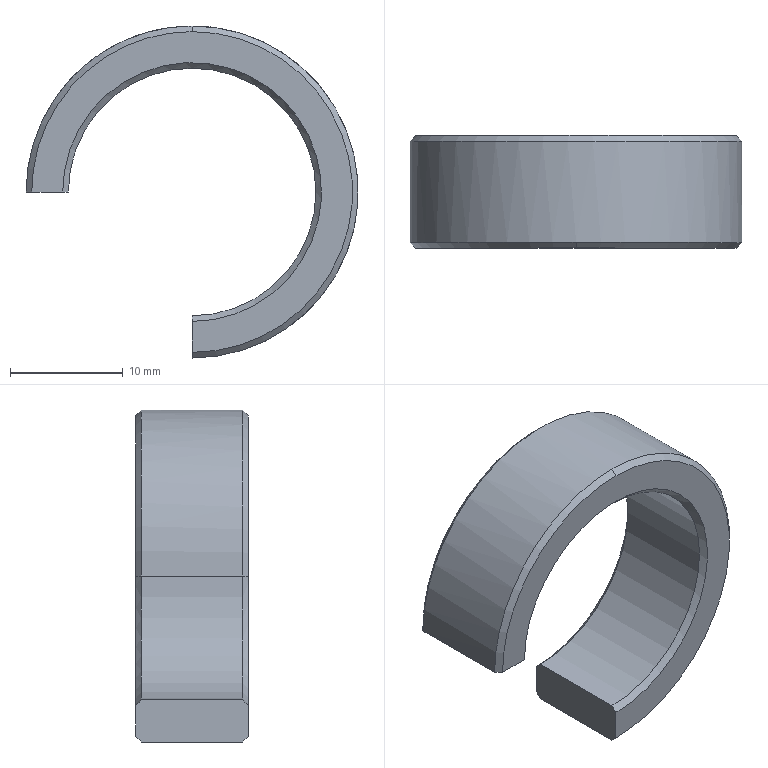Part | STEP file | Cuon T phu H01_3 | 1 solid | 12 faces | box 29.5 x 10 x 29.5 mm | volume 2245 mm3 | cone 6 | plane 4 | cylinder 2 | commonest cylinder face diameters 22 x1 29.5 x1
STEP:
#1=CARTESIAN_POINT('',(0.,0.,0.));
#2=DIRECTION('',(0.,0.,1.));
#3=DIRECTION('',(1.,0.,0.));
#4=AXIS2_PLACEMENT_3D('',#1,#2,#3);
#5=CARTESIAN_POINT('',(0.,10.,-11.5));
#6=VERTEX_POINT('',#5);
#7=CARTESIAN_POINT('',(0.,9.5,-11.));
#8=VERTEX_POINT('',#7);
#9=CARTESIAN_POINT('',(0.,-1.5,0.));
#10=DIRECTION('',(0.,-0.7071,0.7071));
#11=VECTOR('',#10,1.);
#12=LINE('',#9,#11);
#13=CARTESIAN_POINT('',(0.,9.5,0.));
#14=DIRECTION('',(0.,1.,0.));
#15=DIRECTION('',(0.,0.,1.));
#16=AXIS2_PLACEMENT_3D('',#13,#14,#15);
#17=CONICAL_SURFACE('',#16,11.,0.7854);
#18=CARTESIAN_POINT('',(3.142,-11.));
#19=DIRECTION('',(0.,-1.));
#20=VECTOR('',#19,1.);
#21=LINE('',#18,#20);
#22=(GEOMETRIC_REPRESENTATION_CONTEXT(2)PARAMETRIC_REPRESENTATION_CONTEXT()REPRESENTATION_CONTEXT('',''));
#23=DEFINITIONAL_REPRESENTATION('',(#21),#22);
#24=PCURVE('',#17,#23);
#25=CARTESIAN_POINT('',(0.,-63.834,33.935));
#26=DIRECTION('',(-1.,0.,0.));
#27=DIRECTION('',(0.,0.,1.));
#28=AXIS2_PLACEMENT_3D('',#25,#26,#27);
#29=PLANE('',#28);
#30=CARTESIAN_POINT('',(-33.935,62.334));
#31=DIRECTION('',(0.7071,-0.7071));
#32=VECTOR('',#31,1.);
#33=LINE('',#30,#32);
#34=(GEOMETRIC_REPRESENTATION_CONTEXT(2)PARAMETRIC_REPRESENTATION_CONTEXT()REPRESENTATION_CONTEXT('',''));
#35=DEFINITIONAL_REPRESENTATION('',(#33),#34);
#36=PCURVE('',#29,#35);
#37=SURFACE_CURVE('',#12,(#24,#36),.PCURVE_S1.);
#38=EDGE_CURVE('',#6,#8,#37,.T.);
#39=ORIENTED_EDGE('',*,*,#38,.F.);
#40=CARTESIAN_POINT('',(0.,10.,11.5));
#41=VERTEX_POINT('',#40);
#42=CARTESIAN_POINT('',(0.,10.,0.));
#43=DIRECTION('',(0.,-1.,0.));
#44=DIRECTION('',(0.,0.,1.));
#45=AXIS2_PLACEMENT_3D('',#42,#43,#44);
#46=CIRCLE('',#45,11.5);
#47=CARTESIAN_POINT('',(6.283,0.5));
#48=DIRECTION('',(-1.,0.));
#49=VECTOR('',#48,1.);
#50=LINE('',#47,#49);
#51=(GEOMETRIC_REPRESENTATION_CONTEXT(2)PARAMETRIC_REPRESENTATION_CONTEXT()REPRESENTATION_CONTEXT('',''));
#52=DEFINITIONAL_REPRESENTATION('',(#50),#51);
#53=PCURVE('',#17,#52);
#54=CARTESIAN_POINT('',(0.,10.,0.));
#55=DIRECTION('',(0.,1.,0.));
#56=DIRECTION('',(0.,0.,1.));
#57=AXIS2_PLACEMENT_3D('',#54,#55,#56);
#58=PLANE('',#57);
#59=CARTESIAN_POINT('',(11.5,0.));
#60=CARTESIAN_POINT('',(11.5,-19.919));
#61=CARTESIAN_POINT('',(-5.75,-9.959));
#62=CARTESIAN_POINT('',(-23.,0.));
#63=CARTESIAN_POINT('',(-5.75,9.959));
#64=CARTESIAN_POINT('',(11.5,19.919));
#65=CARTESIAN_POINT('',(11.5,0.));
#66=(BOUNDED_CURVE()B_SPLINE_CURVE(2,(#59,#60,#61,#62,#63,#64,#65),.UNSPECIFIED.,.T.,.F.)B_SPLINE_CURVE_WITH_KNOTS((1,2,2,2,2,1),(-2.094,0.,2.094,4.189,6.283,8.378),.UNSPECIFIED.)CURVE()GEOMETRIC_REPRESENTATION_ITEM()RATIONAL_B_SPLINE_CURVE((1.,0.5,1.,0.5,1.,0.5,1.))REPRESENTATION_ITEM(''));
#67=(GEOMETRIC_REPRESENTATION_CONTEXT(2)PARAMETRIC_REPRESENTATION_CONTEXT()REPRESENTATION_CONTEXT('',''));
#68=DEFINITIONAL_REPRESENTATION('',(#66),#67);
#69=PCURVE('',#58,#68);
#70=SURFACE_CURVE('',#46,(#53,#69),.PCURVE_S1.);
#71=EDGE_CURVE('',#6,#41,#70,.T.);
#72=ORIENTED_EDGE('',*,*,#71,.T.);
#73=CARTESIAN_POINT('',(0.,9.5,11.));
#74=VERTEX_POINT('',#73);
#75=CARTESIAN_POINT('',(0.,9.5,11.));
#76=DIRECTION('',(0.,0.7071,0.7071));
#77=VECTOR('',#76,1.);
#78=LINE('',#75,#77);
#79=CARTESIAN_POINT('',(0.,0.));
#80=DIRECTION('',(0.,1.));
#81=VECTOR('',#80,1.);
#82=LINE('',#79,#81);
#83=(GEOMETRIC_REPRESENTATION_CONTEXT(2)PARAMETRIC_REPRESENTATION_CONTEXT()REPRESENTATION_CONTEXT('',''));
#84=DEFINITIONAL_REPRESENTATION('',(#82),#83);
#85=PCURVE('',#17,#84);
#86=CARTESIAN_POINT('',(0.,9.5,0.));
#87=DIRECTION('',(0.,1.,0.));
#88=DIRECTION('',(0.,0.,1.));
#89=AXIS2_PLACEMENT_3D('',#86,#87,#88);
#90=CONICAL_SURFACE('',#89,11.,0.7854);
#91=CARTESIAN_POINT('',(6.283,0.));
#92=DIRECTION('',(0.,1.));
#93=VECTOR('',#92,1.);
#94=LINE('',#91,#93);
#95=(GEOMETRIC_REPRESENTATION_CONTEXT(2)PARAMETRIC_REPRESENTATION_CONTEXT()REPRESENTATION_CONTEXT('',''));
#96=DEFINITIONAL_REPRESENTATION('',(#94),#95);
#97=PCURVE('',#90,#96);
#98=SURFACE_CURVE('',#78,(#85,#97),.PCURVE_S1.);
#99=EDGE_CURVE('',#74,#41,#98,.T.);
#100=ORIENTED_EDGE('',*,*,#99,.F.);
#101=CARTESIAN_POINT('',(0.,9.5,0.));
#102=DIRECTION('',(0.,1.,0.));
#103=DIRECTION('',(0.,0.,1.));
#104=AXIS2_PLACEMENT_3D('',#101,#102,#103);
#105=CIRCLE('',#104,11.);
#106=CARTESIAN_POINT('',(0.,0.));
#107=DIRECTION('',(1.,0.));
#108=VECTOR('',#107,1.);
#109=LINE('',#106,#108);
#110=(GEOMETRIC_REPRESENTATION_CONTEXT(2)PARAMETRIC_REPRESENTATION_CONTEXT()REPRESENTATION_CONTEXT('',''));
#111=DEFINITIONAL_REPRESENTATION('',(#109),#110);
#112=PCURVE('',#17,#111);
#113=CARTESIAN_POINT('',(0.,10.,0.));
#114=DIRECTION('',(0.,-1.,0.));
#115=DIRECTION('',(0.,0.,-1.));
#116=AXIS2_PLACEMENT_3D('',#113,#114,#115);
#117=CYLINDRICAL_SURFACE('',#116,11.);
#118=CARTESIAN_POINT('',(3.142,0.5));
#119=DIRECTION('',(-1.,0.));
#120=VECTOR('',#119,1.);
#121=LINE('',#118,#120);
#122=(GEOMETRIC_REPRESENTATION_CONTEXT(2)PARAMETRIC_REPRESENTATION_CONTEXT()REPRESENTATION_CONTEXT('',''));
#123=DEFINITIONAL_REPRESENTATION('',(#121),#122);
#124=PCURVE('',#117,#123);
#125=SURFACE_CURVE('',#105,(#112,#124),.PCURVE_S1.);
#126=EDGE_CURVE('',#74,#8,#125,.T.);
#127=ORIENTED_EDGE('',*,*,#126,.T.);
#128=EDGE_LOOP('',(#39,#72,#100,#127));
#129=FACE_BOUND('',#128,.F.);
#130=ADVANCED_FACE('',(#129),#17,.F.);
#131=CARTESIAN_POINT('',(0.,0.,14.25));
#132=VERTEX_POINT('',#131);
#133=CARTESIAN_POINT('',(-14.25,0.,0.));
#134=VERTEX_POINT('',#133);
#135=CARTESIAN_POINT('',(0.,0.,0.));
#136=DIRECTION('',(0.,-1.,0.));
#137=DIRECTION('',(0.,0.,1.));
#138=AXIS2_PLACEMENT_3D('',#135,#136,#137);
#139=CIRCLE('',#138,14.25);
#140=CARTESIAN_POINT('',(0.,0.5,0.));
#141=DIRECTION('',(0.,1.,0.));
#142=DIRECTION('',(0.,0.,1.));
#143=AXIS2_PLACEMENT_3D('',#140,#141,#142);
#144=CONICAL_SURFACE('',#143,14.75,0.7854);
#145=CARTESIAN_POINT('',(6.283,-0.5));
#146=DIRECTION('',(-1.,0.));
#147=VECTOR('',#146,1.);
#148=LINE('',#145,#147);
#149=(GEOMETRIC_REPRESENTATION_CONTEXT(2)PARAMETRIC_REPRESENTATION_CONTEXT()REPRESENTATION_CONTEXT('',''));
#150=DEFINITIONAL_REPRESENTATION('',(#148),#149);
#151=PCURVE('',#144,#150);
#152=CARTESIAN_POINT('',(0.,0.,0.));
#153=DIRECTION('',(0.,1.,0.));
#154=DIRECTION('',(0.,0.,1.));
#155=AXIS2_PLACEMENT_3D('',#152,#153,#154);
#156=PLANE('',#155);
#157=CARTESIAN_POINT('',(14.25,0.));
#158=CARTESIAN_POINT('',(14.25,-24.682));
#159=CARTESIAN_POINT('',(-7.125,-12.341));
#160=CARTESIAN_POINT('',(-28.5,0.));
#161=CARTESIAN_POINT('',(-7.125,12.341));
#162=CARTESIAN_POINT('',(14.25,24.682));
#163=CARTESIAN_POINT('',(14.25,0.));
#164=(BOUNDED_CURVE()B_SPLINE_CURVE(2,(#157,#158,#159,#160,#161,#162,#163),.UNSPECIFIED.,.T.,.F.)B_SPLINE_CURVE_WITH_KNOTS((1,2,2,2,2,1),(-2.094,0.,2.094,4.189,6.283,8.378),.UNSPECIFIED.)CURVE()GEOMETRIC_REPRESENTATION_ITEM()RATIONAL_B_SPLINE_CURVE((1.,0.5,1.,0.5,1.,0.5,1.))REPRESENTATION_ITEM(''));
#165=(GEOMETRIC_REPRESENTATION_CONTEXT(2)PARAMETRIC_REPRESENTATION_CONTEXT()REPRESENTATION_CONTEXT('',''));
#166=DEFINITIONAL_REPRESENTATION('',(#164),#165);
#167=PCURVE('',#156,#166);
#168=SURFACE_CURVE('',#139,(#151,#167),.PCURVE_S1.);
#169=EDGE_CURVE('',#132,#134,#168,.T.);
#170=ORIENTED_EDGE('',*,*,#169,.F.);
#171=CARTESIAN_POINT('',(0.,0.5,14.75));
#172=VERTEX_POINT('',#171);
#173=CARTESIAN_POINT('',(0.,0.5,14.75));
#174=DIRECTION('',(0.,0.7071,0.7071));
#175=VECTOR('',#174,1.);
#176=LINE('',#173,#175);
#177=CARTESIAN_POINT('',(6.283,0.));
#178=DIRECTION('',(0.,1.));
#179=VECTOR('',#178,1.);
#180=LINE('',#177,#179);
#181=(GEOMETRIC_REPRESENTATION_CONTEXT(2)PARAMETRIC_REPRESENTATION_CONTEXT()REPRESENTATION_CONTEXT('',''));
#182=DEFINITIONAL_REPRESENTATION('',(#180),#181);
#183=PCURVE('',#144,#182);
#184=CARTESIAN_POINT('',(0.,0.5,0.));
#185=DIRECTION('',(0.,1.,0.));
#186=DIRECTION('',(0.,0.,1.));
#187=AXIS2_PLACEMENT_3D('',#184,#185,#186);
#188=CONICAL_SURFACE('',#187,14.75,0.7854);
#189=CARTESIAN_POINT('',(0.,0.));
#190=DIRECTION('',(0.,1.));
#191=VECTOR('',#190,1.);
#192=LINE('',#189,#191);
#193=(GEOMETRIC_REPRESENTATION_CONTEXT(2)PARAMETRIC_REPRESENTATION_CONTEXT()REPRESENTATION_CONTEXT('',''));
#194=DEFINITIONAL_REPRESENTATION('',(#192),#193);
#195=PCURVE('',#188,#194);
#196=SURFACE_CURVE('',#176,(#183,#195),.PCURVE_S1.);
#197=EDGE_CURVE('',#132,#172,#196,.T.);
#198=ORIENTED_EDGE('',*,*,#197,.T.);
#199=CARTESIAN_POINT('',(-14.75,0.5,0.));
#200=VERTEX_POINT('',#199);
#201=CARTESIAN_POINT('',(0.,0.5,0.));
#202=DIRECTION('',(0.,1.,0.));
#203=DIRECTION('',(0.,0.,1.));
#204=AXIS2_PLACEMENT_3D('',#201,#202,#203);
#205=CIRCLE('',#204,14.75);
#206=CARTESIAN_POINT('',(0.,0.));
#207=DIRECTION('',(1.,0.));
#208=VECTOR('',#207,1.);
#209=LINE('',#206,#208);
#210=(GEOMETRIC_REPRESENTATION_CONTEXT(2)PARAMETRIC_REPRESENTATION_CONTEXT()REPRESENTATION_CONTEXT('',''));
#211=DEFINITIONAL_REPRESENTATION('',(#209),#210);
#212=PCURVE('',#144,#211);
#213=CARTESIAN_POINT('',(0.,10.,0.));
#214=DIRECTION('',(0.,-1.,0.));
#215=DIRECTION('',(0.,0.,-1.));
#216=AXIS2_PLACEMENT_3D('',#213,#214,#215);
#217=CYLINDRICAL_SURFACE('',#216,14.75);
#218=CARTESIAN_POINT('',(9.425,9.5));
#219=DIRECTION('',(-1.,0.));
#220=VECTOR('',#219,1.);
#221=LINE('',#218,#220);
#222=(GEOMETRIC_REPRESENTATION_CONTEXT(2)PARAMETRIC_REPRESENTATION_CONTEXT()REPRESENTATION_CONTEXT('',''));
#223=DEFINITIONAL_REPRESENTATION('',(#221),#222);
#224=PCURVE('',#217,#223);
#225=SURFACE_CURVE('',#205,(#212,#224),.PCURVE_S1.);
#226=EDGE_CURVE('',#200,#172,#225,.T.);
#227=ORIENTED_EDGE('',*,*,#226,.F.);
#228=CARTESIAN_POINT('',(0.,-14.25,0.));
#229=DIRECTION('',(-0.7071,0.7071,0.));
#230=VECTOR('',#229,1.);
#231=LINE('',#228,#230);
#232=CARTESIAN_POINT('',(4.712,-14.75));
#233=DIRECTION('',(0.,1.));
#234=VECTOR('',#233,1.);
#235=LINE('',#232,#234);
#236=(GEOMETRIC_REPRESENTATION_CONTEXT(2)PARAMETRIC_REPRESENTATION_CONTEXT()REPRESENTATION_CONTEXT('',''));
#237=DEFINITIONAL_REPRESENTATION('',(#235),#236);
#238=PCURVE('',#144,#237);
#239=CARTESIAN_POINT('',(0.,-52.57,0.));
#240=DIRECTION('',(0.,0.,1.));
#241=DIRECTION('',(1.,0.,0.));
#242=AXIS2_PLACEMENT_3D('',#239,#240,#241);
#243=PLANE('',#242);
#244=CARTESIAN_POINT('',(0.,38.32));
#245=DIRECTION('',(-0.7071,0.7071));
#246=VECTOR('',#245,1.);
#247=LINE('',#244,#246);
#248=(GEOMETRIC_REPRESENTATION_CONTEXT(2)PARAMETRIC_REPRESENTATION_CONTEXT()REPRESENTATION_CONTEXT('',''));
#249=DEFINITIONAL_REPRESENTATION('',(#247),#248);
#250=PCURVE('',#243,#249);
#251=SURFACE_CURVE('',#231,(#238,#250),.PCURVE_S1.);
#252=EDGE_CURVE('',#134,#200,#251,.T.);
#253=ORIENTED_EDGE('',*,*,#252,.F.);
#254=EDGE_LOOP('',(#170,#198,#227,#253));
#255=FACE_BOUND('',#254,.T.);
#256=ADVANCED_FACE('',(#255),#144,.T.);
#257=CARTESIAN_POINT('',(-14.25,10.,0.));
#258=VERTEX_POINT('',#257);
#259=CARTESIAN_POINT('',(-11.5,10.,0.));
#260=VERTEX_POINT('',#259);
#261=CARTESIAN_POINT('',(0.,10.,0.));
#262=DIRECTION('',(1.,0.,0.));
#263=VECTOR('',#262,1.);
#264=LINE('',#261,#263);
#265=CARTESIAN_POINT('',(0.,0.));
#266=DIRECTION('',(0.,1.));
#267=VECTOR('',#266,1.);
#268=LINE('',#265,#267);
#269=(GEOMETRIC_REPRESENTATION_CONTEXT(2)PARAMETRIC_REPRESENTATION_CONTEXT()REPRESENTATION_CONTEXT('',''));
#270=DEFINITIONAL_REPRESENTATION('',(#268),#269);
#271=PCURVE('',#58,#270);
#272=CARTESIAN_POINT('',(0.,62.57));
#273=DIRECTION('',(1.,0.));
#274=VECTOR('',#273,1.);
#275=LINE('',#272,#274);
#276=(GEOMETRIC_REPRESENTATION_CONTEXT(2)PARAMETRIC_REPRESENTATION_CONTEXT()REPRESENTATION_CONTEXT('',''));
#277=DEFINITIONAL_REPRESENTATION('',(#275),#276);
#278=PCURVE('',#243,#277);
#279=SURFACE_CURVE('',#264,(#271,#278),.PCURVE_S1.);
#280=EDGE_CURVE('',#258,#260,#279,.T.);
#281=ORIENTED_EDGE('',*,*,#280,.F.);
#282=CARTESIAN_POINT('',(0.,10.,-14.25));
#283=VERTEX_POINT('',#282);
#284=CARTESIAN_POINT('',(0.,10.,0.));
#285=DIRECTION('',(0.,1.,0.));
#286=DIRECTION('',(0.,0.,1.));
#287=AXIS2_PLACEMENT_3D('',#284,#285,#286);
#288=CIRCLE('',#287,14.25);
#289=CARTESIAN_POINT('',(0.,0.));
#290=DIRECTION('',(1.,0.));
#291=AXIS2_PLACEMENT_2D('',#289,#290);
#292=CIRCLE('',#291,14.25);
#293=(GEOMETRIC_REPRESENTATION_CONTEXT(2)PARAMETRIC_REPRESENTATION_CONTEXT()REPRESENTATION_CONTEXT('',''));
#294=DEFINITIONAL_REPRESENTATION('',(#292),#293);
#295=PCURVE('',#58,#294);
#296=CARTESIAN_POINT('',(0.,10.,0.));
#297=DIRECTION('',(0.,-1.,0.));
#298=DIRECTION('',(0.,0.,-1.));
#299=AXIS2_PLACEMENT_3D('',#296,#297,#298);
#300=CONICAL_SURFACE('',#299,14.25,0.7854);
#301=CARTESIAN_POINT('',(9.425,0.));
#302=DIRECTION('',(-1.,0.));
#303=VECTOR('',#302,1.);
#304=LINE('',#301,#303);
#305=(GEOMETRIC_REPRESENTATION_CONTEXT(2)PARAMETRIC_REPRESENTATION_CONTEXT()REPRESENTATION_CONTEXT('',''));
#306=DEFINITIONAL_REPRESENTATION('',(#304),#305);
#307=PCURVE('',#300,#306);
#308=SURFACE_CURVE('',#288,(#295,#307),.PCURVE_S1.);
#309=EDGE_CURVE('',#258,#283,#308,.T.);
#310=ORIENTED_EDGE('',*,*,#309,.T.);
#311=CARTESIAN_POINT('',(0.,10.,0.));
#312=DIRECTION('',(0.,0.,1.));
#313=VECTOR('',#312,1.);
#314=LINE('',#311,#313);
#315=CARTESIAN_POINT('',(0.,0.));
#316=DIRECTION('',(1.,0.));
#317=VECTOR('',#316,1.);
#318=LINE('',#315,#317);
#319=(GEOMETRIC_REPRESENTATION_CONTEXT(2)PARAMETRIC_REPRESENTATION_CONTEXT()REPRESENTATION_CONTEXT('',''));
#320=DEFINITIONAL_REPRESENTATION('',(#318),#319);
#321=PCURVE('',#58,#320);
#322=CARTESIAN_POINT('',(-33.935,73.834));
#323=DIRECTION('',(1.,0.));
#324=VECTOR('',#323,1.);
#325=LINE('',#322,#324);
#326=(GEOMETRIC_REPRESENTATION_CONTEXT(2)PARAMETRIC_REPRESENTATION_CONTEXT()REPRESENTATION_CONTEXT('',''));
#327=DEFINITIONAL_REPRESENTATION('',(#325),#326);
#328=PCURVE('',#29,#327);
#329=SURFACE_CURVE('',#314,(#321,#328),.PCURVE_S1.);
#330=EDGE_CURVE('',#283,#6,#329,.T.);
#331=ORIENTED_EDGE('',*,*,#330,.T.);
#332=ORIENTED_EDGE('',*,*,#71,.T.);
#333=CARTESIAN_POINT('',(0.,10.,0.));
#334=DIRECTION('',(0.,-1.,0.));
#335=DIRECTION('',(0.,0.,1.));
#336=AXIS2_PLACEMENT_3D('',#333,#334,#335);
#337=CIRCLE('',#336,11.5);
#338=CARTESIAN_POINT('',(11.5,0.));
#339=CARTESIAN_POINT('',(11.5,-19.919));
#340=CARTESIAN_POINT('',(-5.75,-9.959));
#341=CARTESIAN_POINT('',(-23.,0.));
#342=CARTESIAN_POINT('',(-5.75,9.959));
#343=CARTESIAN_POINT('',(11.5,19.919));
#344=CARTESIAN_POINT('',(11.5,0.));
#345=(BOUNDED_CURVE()B_SPLINE_CURVE(2,(#338,#339,#340,#341,#342,#343,#344),.UNSPECIFIED.,.T.,.F.)B_SPLINE_CURVE_WITH_KNOTS((1,2,2,2,2,1),(-2.094,0.,2.094,4.189,6.283,8.378),.UNSPECIFIED.)CURVE()GEOMETRIC_REPRESENTATION_ITEM()RATIONAL_B_SPLINE_CURVE((1.,0.5,1.,0.5,1.,0.5,1.))REPRESENTATION_ITEM(''));
#346=(GEOMETRIC_REPRESENTATION_CONTEXT(2)PARAMETRIC_REPRESENTATION_CONTEXT()REPRESENTATION_CONTEXT('',''));
#347=DEFINITIONAL_REPRESENTATION('',(#345),#346);
#348=PCURVE('',#58,#347);
#349=CARTESIAN_POINT('',(6.283,0.5));
#350=DIRECTION('',(-1.,0.));
#351=VECTOR('',#350,1.);
#352=LINE('',#349,#351);
#353=(GEOMETRIC_REPRESENTATION_CONTEXT(2)PARAMETRIC_REPRESENTATION_CONTEXT()REPRESENTATION_CONTEXT('',''));
#354=DEFINITIONAL_REPRESENTATION('',(#352),#353);
#355=PCURVE('',#90,#354);
#356=SURFACE_CURVE('',#337,(#348,#355),.PCURVE_S1.);
#357=EDGE_CURVE('',#41,#260,#356,.T.);
#358=ORIENTED_EDGE('',*,*,#357,.T.);
#359=EDGE_LOOP('',(#281,#310,#331,#332,#358));
#360=FACE_BOUND('',#359,.T.);
#361=ADVANCED_FACE('',(#360),#58,.T.);
#362=CARTESIAN_POINT('',(0.,0.,-14.25));
#363=VERTEX_POINT('',#362);
#364=CARTESIAN_POINT('',(0.,0.,0.));
#365=DIRECTION('',(0.,-1.,0.));
#366=DIRECTION('',(0.,0.,1.));
#367=AXIS2_PLACEMENT_3D('',#364,#365,#366);
#368=CIRCLE('',#367,14.25);
#369=CARTESIAN_POINT('',(14.25,0.));
#370=CARTESIAN_POINT('',(14.25,-24.682));
#371=CARTESIAN_POINT('',(-7.125,-12.341));
#372=CARTESIAN_POINT('',(-28.5,0.));
#373=CARTESIAN_POINT('',(-7.125,12.341));
#374=CARTESIAN_POINT('',(14.25,24.682));
#375=CARTESIAN_POINT('',(14.25,0.));
#376=(BOUNDED_CURVE()B_SPLINE_CURVE(2,(#369,#370,#371,#372,#373,#374,#375),.UNSPECIFIED.,.T.,.F.)B_SPLINE_CURVE_WITH_KNOTS((1,2,2,2,2,1),(-2.094,0.,2.094,4.189,6.283,8.378),.UNSPECIFIED.)CURVE()GEOMETRIC_REPRESENTATION_ITEM()RATIONAL_B_SPLINE_CURVE((1.,0.5,1.,0.5,1.,0.5,1.))REPRESENTATION_ITEM(''));
#377=(GEOMETRIC_REPRESENTATION_CONTEXT(2)PARAMETRIC_REPRESENTATION_CONTEXT()REPRESENTATION_CONTEXT('',''));
#378=DEFINITIONAL_REPRESENTATION('',(#376),#377);
#379=PCURVE('',#156,#378);
#380=CARTESIAN_POINT('',(6.283,-0.5));
#381=DIRECTION('',(-1.,0.));
#382=VECTOR('',#381,1.);
#383=LINE('',#380,#382);
#384=(GEOMETRIC_REPRESENTATION_CONTEXT(2)PARAMETRIC_REPRESENTATION_CONTEXT()REPRESENTATION_CONTEXT('',''));
#385=DEFINITIONAL_REPRESENTATION('',(#383),#384);
#386=PCURVE('',#188,#385);
#387=SURFACE_CURVE('',#368,(#379,#386),.PCURVE_S1.);
#388=EDGE_CURVE('',#363,#132,#387,.T.);
#389=ORIENTED_EDGE('',*,*,#388,.T.);
#390=ORIENTED_EDGE('',*,*,#169,.T.);
#391=CARTESIAN_POINT('',(-11.5,0.,0.));
#392=VERTEX_POINT('',#391);
#393=CARTESIAN_POINT('',(0.,0.,0.));
#394=DIRECTION('',(1.,0.,0.));
#395=VECTOR('',#394,1.);
#396=LINE('',#393,#395);
#397=CARTESIAN_POINT('',(0.,0.));
#398=DIRECTION('',(0.,1.));
#399=VECTOR('',#398,1.);
#400=LINE('',#397,#399);
#401=(GEOMETRIC_REPRESENTATION_CONTEXT(2)PARAMETRIC_REPRESENTATION_CONTEXT()REPRESENTATION_CONTEXT('',''));
#402=DEFINITIONAL_REPRESENTATION('',(#400),#401);
#403=PCURVE('',#156,#402);
#404=CARTESIAN_POINT('',(0.,52.57));
#405=DIRECTION('',(1.,0.));
#406=VECTOR('',#405,1.);
#407=LINE('',#404,#406);
#408=(GEOMETRIC_REPRESENTATION_CONTEXT(2)PARAMETRIC_REPRESENTATION_CONTEXT()REPRESENTATION_CONTEXT('',''));
#409=DEFINITIONAL_REPRESENTATION('',(#407),#408);
#410=PCURVE('',#243,#409);
#411=SURFACE_CURVE('',#396,(#403,#410),.PCURVE_S1.);
#412=EDGE_CURVE('',#134,#392,#411,.T.);
#413=ORIENTED_EDGE('',*,*,#412,.T.);
#414=CARTESIAN_POINT('',(0.,0.,-11.5));
#415=VERTEX_POINT('',#414);
#416=CARTESIAN_POINT('',(0.,0.,0.));
#417=DIRECTION('',(0.,1.,0.));
#418=DIRECTION('',(0.,0.,1.));
#419=AXIS2_PLACEMENT_3D('',#416,#417,#418);
#420=CIRCLE('',#419,11.5);
#421=CARTESIAN_POINT('',(0.,0.));
#422=DIRECTION('',(1.,0.));
#423=AXIS2_PLACEMENT_2D('',#421,#422);
#424=CIRCLE('',#423,11.5);
#425=(GEOMETRIC_REPRESENTATION_CONTEXT(2)PARAMETRIC_REPRESENTATION_CONTEXT()REPRESENTATION_CONTEXT('',''));
#426=DEFINITIONAL_REPRESENTATION('',(#424),#425);
#427=PCURVE('',#156,#426);
#428=CARTESIAN_POINT('',(0.,0.,0.));
#429=DIRECTION('',(0.,-1.,0.));
#430=DIRECTION('',(0.,0.,-1.));
#431=AXIS2_PLACEMENT_3D('',#428,#429,#430);
#432=CONICAL_SURFACE('',#431,11.5,0.7854);
#433=CARTESIAN_POINT('',(9.425,0.));
#434=DIRECTION('',(-1.,0.));
#435=VECTOR('',#434,1.);
#436=LINE('',#433,#435);
#437=(GEOMETRIC_REPRESENTATION_CONTEXT(2)PARAMETRIC_REPRESENTATION_CONTEXT()REPRESENTATION_CONTEXT('',''));
#438=DEFINITIONAL_REPRESENTATION('',(#436),#437);
#439=PCURVE('',#432,#438);
#440=SURFACE_CURVE('',#420,(#427,#439),.PCURVE_S1.);
#441=EDGE_CURVE('',#392,#415,#440,.T.);
#442=ORIENTED_EDGE('',*,*,#441,.T.);
#443=CARTESIAN_POINT('',(0.,0.,0.));
#444=DIRECTION('',(0.,0.,1.));
#445=VECTOR('',#444,1.);
#446=LINE('',#443,#445);
#447=CARTESIAN_POINT('',(0.,0.));
#448=DIRECTION('',(1.,0.));
#449=VECTOR('',#448,1.);
#450=LINE('',#447,#449);
#451=(GEOMETRIC_REPRESENTATION_CONTEXT(2)PARAMETRIC_REPRESENTATION_CONTEXT()REPRESENTATION_CONTEXT('',''));
#452=DEFINITIONAL_REPRESENTATION('',(#450),#451);
#453=PCURVE('',#156,#452);
#454=CARTESIAN_POINT('',(-33.935,63.834));
#455=DIRECTION('',(1.,0.));
#456=VECTOR('',#455,1.);
#457=LINE('',#454,#456);
#458=(GEOMETRIC_REPRESENTATION_CONTEXT(2)PARAMETRIC_REPRESENTATION_CONTEXT()REPRESENTATION_CONTEXT('',''));
#459=DEFINITIONAL_REPRESENTATION('',(#457),#458);
#460=PCURVE('',#29,#459);
#461=SURFACE_CURVE('',#446,(#453,#460),.PCURVE_S1.);
#462=EDGE_CURVE('',#363,#415,#461,.T.);
#463=ORIENTED_EDGE('',*,*,#462,.F.);
#464=EDGE_LOOP('',(#389,#390,#413,#442,#463));
#465=FACE_BOUND('',#464,.T.);
#466=ADVANCED_FACE('',(#465),#156,.F.);
#467=CARTESIAN_POINT('',(0.,9.5,-14.75));
#468=VERTEX_POINT('',#467);
#469=CARTESIAN_POINT('',(-14.75,9.5,0.));
#470=VERTEX_POINT('',#469);
#471=CARTESIAN_POINT('',(0.,9.5,0.));
#472=DIRECTION('',(0.,-1.,0.));
#473=DIRECTION('',(0.,0.,1.));
#474=AXIS2_PLACEMENT_3D('',#471,#472,#473);
#475=CIRCLE('',#474,14.75);
#476=CARTESIAN_POINT('',(-3.142,0.5));
#477=DIRECTION('',(1.,0.));
#478=VECTOR('',#477,1.);
#479=LINE('',#476,#478);
#480=(GEOMETRIC_REPRESENTATION_CONTEXT(2)PARAMETRIC_REPRESENTATION_CONTEXT()REPRESENTATION_CONTEXT('',''));
#481=DEFINITIONAL_REPRESENTATION('',(#479),#480);
#482=PCURVE('',#217,#481);
#483=CARTESIAN_POINT('',(-3.142,0.5));
#484=DIRECTION('',(1.,0.));
#485=VECTOR('',#484,1.);
#486=LINE('',#483,#485);
#487=(GEOMETRIC_REPRESENTATION_CONTEXT(2)PARAMETRIC_REPRESENTATION_CONTEXT()REPRESENTATION_CONTEXT('',''));
#488=DEFINITIONAL_REPRESENTATION('',(#486),#487);
#489=PCURVE('',#300,#488);
#490=SURFACE_CURVE('',#475,(#482,#489),.PCURVE_S1.);
#491=EDGE_CURVE('',#468,#470,#490,.T.);
#492=ORIENTED_EDGE('',*,*,#491,.T.);
#493=CARTESIAN_POINT('',(-14.75,10.,0.));
#494=DIRECTION('',(0.,-1.,0.));
#495=VECTOR('',#494,1.);
#496=LINE('',#493,#495);
#497=CARTESIAN_POINT('',(4.712,0.));
#498=DIRECTION('',(0.,1.));
#499=VECTOR('',#498,1.);
#500=LINE('',#497,#499);
#501=(GEOMETRIC_REPRESENTATION_CONTEXT(2)PARAMETRIC_REPRESENTATION_CONTEXT()REPRESENTATION_CONTEXT('',''));
#502=DEFINITIONAL_REPRESENTATION('',(#500),#501);
#503=PCURVE('',#217,#502);
#504=CARTESIAN_POINT('',(-14.75,62.57));
#505=DIRECTION('',(0.,-1.));
#506=VECTOR('',#505,1.);
#507=LINE('',#504,#506);
#508=(GEOMETRIC_REPRESENTATION_CONTEXT(2)PARAMETRIC_REPRESENTATION_CONTEXT()REPRESENTATION_CONTEXT('',''));
#509=DEFINITIONAL_REPRESENTATION('',(#507),#508);
#510=PCURVE('',#243,#509);
#511=SURFACE_CURVE('',#496,(#503,#510),.PCURVE_S1.);
#512=EDGE_CURVE('',#470,#200,#511,.T.);
#513=ORIENTED_EDGE('',*,*,#512,.T.);
#514=ORIENTED_EDGE('',*,*,#226,.T.);
#515=CARTESIAN_POINT('',(0.,0.5,-14.75));
#516=VERTEX_POINT('',#515);
#517=CARTESIAN_POINT('',(0.,0.5,0.));
#518=DIRECTION('',(0.,1.,0.));
#519=DIRECTION('',(0.,0.,1.));
#520=AXIS2_PLACEMENT_3D('',#517,#518,#519);
#521=CIRCLE('',#520,14.75);
#522=CARTESIAN_POINT('',(3.142,9.5));
#523=DIRECTION('',(-1.,0.));
#524=VECTOR('',#523,1.);
#525=LINE('',#522,#524);
#526=(GEOMETRIC_REPRESENTATION_CONTEXT(2)PARAMETRIC_REPRESENTATION_CONTEXT()REPRESENTATION_CONTEXT('',''));
#527=DEFINITIONAL_REPRESENTATION('',(#525),#526);
#528=PCURVE('',#217,#527);
#529=CARTESIAN_POINT('',(0.,0.));
#530=DIRECTION('',(1.,0.));
#531=VECTOR('',#530,1.);
#532=LINE('',#529,#531);
#533=(GEOMETRIC_REPRESENTATION_CONTEXT(2)PARAMETRIC_REPRESENTATION_CONTEXT()REPRESENTATION_CONTEXT('',''));
#534=DEFINITIONAL_REPRESENTATION('',(#532),#533);
#535=PCURVE('',#188,#534);
#536=SURFACE_CURVE('',#521,(#528,#535),.PCURVE_S1.);
#537=EDGE_CURVE('',#172,#516,#536,.T.);
#538=ORIENTED_EDGE('',*,*,#537,.T.);
#539=CARTESIAN_POINT('',(0.,10.,-14.75));
#540=DIRECTION('',(0.,-1.,0.));
#541=VECTOR('',#540,1.);
#542=LINE('',#539,#541);
#543=CARTESIAN_POINT('',(0.,0.));
#544=DIRECTION('',(0.,1.));
#545=VECTOR('',#544,1.);
#546=LINE('',#543,#545);
#547=(GEOMETRIC_REPRESENTATION_CONTEXT(2)PARAMETRIC_REPRESENTATION_CONTEXT()REPRESENTATION_CONTEXT('',''));
#548=DEFINITIONAL_REPRESENTATION('',(#546),#547);
#549=PCURVE('',#217,#548);
#550=CARTESIAN_POINT('',(-48.685,73.834));
#551=DIRECTION('',(0.,-1.));
#552=VECTOR('',#551,1.);
#553=LINE('',#550,#552);
#554=(GEOMETRIC_REPRESENTATION_CONTEXT(2)PARAMETRIC_REPRESENTATION_CONTEXT()REPRESENTATION_CONTEXT('',''));
#555=DEFINITIONAL_REPRESENTATION('',(#553),#554);
#556=PCURVE('',#29,#555);
#557=SURFACE_CURVE('',#542,(#549,#556),.PCURVE_S1.);
#558=EDGE_CURVE('',#468,#516,#557,.T.);
#559=ORIENTED_EDGE('',*,*,#558,.F.);
#560=EDGE_LOOP('',(#492,#513,#514,#538,#559));
#561=FACE_BOUND('',#560,.T.);
#562=ADVANCED_FACE('',(#561),#217,.T.);
#563=CARTESIAN_POINT('',(0.,0.5,-11.));
#564=VERTEX_POINT('',#563);
#565=CARTESIAN_POINT('',(-11.,0.5,0.));
#566=VERTEX_POINT('',#565);
#567=CARTESIAN_POINT('',(0.,0.5,0.));
#568=DIRECTION('',(0.,-1.,0.));
#569=DIRECTION('',(0.,0.,1.));
#570=AXIS2_PLACEMENT_3D('',#567,#568,#569);
#571=CIRCLE('',#570,11.);
#572=CARTESIAN_POINT('',(-3.142,9.5));
#573=DIRECTION('',(1.,0.));
#574=VECTOR('',#573,1.);
#575=LINE('',#572,#574);
#576=(GEOMETRIC_REPRESENTATION_CONTEXT(2)PARAMETRIC_REPRESENTATION_CONTEXT()REPRESENTATION_CONTEXT('',''));
#577=DEFINITIONAL_REPRESENTATION('',(#575),#576);
#578=PCURVE('',#117,#577);
#579=CARTESIAN_POINT('',(-3.142,-0.5));
#580=DIRECTION('',(1.,0.));
#581=VECTOR('',#580,1.);
#582=LINE('',#579,#581);
#583=(GEOMETRIC_REPRESENTATION_CONTEXT(2)PARAMETRIC_REPRESENTATION_CONTEXT()REPRESENTATION_CONTEXT('',''));
#584=DEFINITIONAL_REPRESENTATION('',(#582),#583);
#585=PCURVE('',#432,#584);
#586=SURFACE_CURVE('',#571,(#578,#585),.PCURVE_S1.);
#587=EDGE_CURVE('',#564,#566,#586,.T.);
#588=ORIENTED_EDGE('',*,*,#587,.F.);
#589=CARTESIAN_POINT('',(0.,10.,-11.));
#590=DIRECTION('',(0.,-1.,0.));
#591=VECTOR('',#590,1.);
#592=LINE('',#589,#591);
#593=CARTESIAN_POINT('',(0.,0.));
#594=DIRECTION('',(0.,1.));
#595=VECTOR('',#594,1.);
#596=LINE('',#593,#595);
#597=(GEOMETRIC_REPRESENTATION_CONTEXT(2)PARAMETRIC_REPRESENTATION_CONTEXT()REPRESENTATION_CONTEXT('',''));
#598=DEFINITIONAL_REPRESENTATION('',(#596),#597);
#599=PCURVE('',#117,#598);
#600=CARTESIAN_POINT('',(-44.935,73.834));
#601=DIRECTION('',(0.,-1.));
#602=VECTOR('',#601,1.);
#603=LINE('',#600,#602);
#604=(GEOMETRIC_REPRESENTATION_CONTEXT(2)PARAMETRIC_REPRESENTATION_CONTEXT()REPRESENTATION_CONTEXT('',''));
#605=DEFINITIONAL_REPRESENTATION('',(#603),#604);
#606=PCURVE('',#29,#605);
#607=SURFACE_CURVE('',#592,(#599,#606),.PCURVE_S1.);
#608=EDGE_CURVE('',#8,#564,#607,.T.);
#609=ORIENTED_EDGE('',*,*,#608,.F.);
#610=ORIENTED_EDGE('',*,*,#126,.F.);
#611=CARTESIAN_POINT('',(-11.,9.5,0.));
#612=VERTEX_POINT('',#611);
#613=CARTESIAN_POINT('',(0.,9.5,0.));
#614=DIRECTION('',(0.,1.,0.));
#615=DIRECTION('',(0.,0.,1.));
#616=AXIS2_PLACEMENT_3D('',#613,#614,#615);
#617=CIRCLE('',#616,11.);
#618=CARTESIAN_POINT('',(9.425,0.5));
#619=DIRECTION('',(-1.,0.));
#620=VECTOR('',#619,1.);
#621=LINE('',#618,#620);
#622=(GEOMETRIC_REPRESENTATION_CONTEXT(2)PARAMETRIC_REPRESENTATION_CONTEXT()REPRESENTATION_CONTEXT('',''));
#623=DEFINITIONAL_REPRESENTATION('',(#621),#622);
#624=PCURVE('',#117,#623);
#625=CARTESIAN_POINT('',(0.,0.));
#626=DIRECTION('',(1.,0.));
#627=VECTOR('',#626,1.);
#628=LINE('',#625,#627);
#629=(GEOMETRIC_REPRESENTATION_CONTEXT(2)PARAMETRIC_REPRESENTATION_CONTEXT()REPRESENTATION_CONTEXT('',''));
#630=DEFINITIONAL_REPRESENTATION('',(#628),#629);
#631=PCURVE('',#90,#630);
#632=SURFACE_CURVE('',#617,(#624,#631),.PCURVE_S1.);
#633=EDGE_CURVE('',#612,#74,#632,.T.);
#634=ORIENTED_EDGE('',*,*,#633,.F.);
#635=CARTESIAN_POINT('',(-11.,10.,0.));
#636=DIRECTION('',(0.,-1.,0.));
#637=VECTOR('',#636,1.);
#638=LINE('',#635,#637);
#639=CARTESIAN_POINT('',(4.712,0.));
#640=DIRECTION('',(0.,1.));
#641=VECTOR('',#640,1.);
#642=LINE('',#639,#641);
#643=(GEOMETRIC_REPRESENTATION_CONTEXT(2)PARAMETRIC_REPRESENTATION_CONTEXT()REPRESENTATION_CONTEXT('',''));
#644=DEFINITIONAL_REPRESENTATION('',(#642),#643);
#645=PCURVE('',#117,#644);
#646=CARTESIAN_POINT('',(-11.,62.57));
#647=DIRECTION('',(0.,-1.));
#648=VECTOR('',#647,1.);
#649=LINE('',#646,#648);
#650=(GEOMETRIC_REPRESENTATION_CONTEXT(2)PARAMETRIC_REPRESENTATION_CONTEXT()REPRESENTATION_CONTEXT('',''));
#651=DEFINITIONAL_REPRESENTATION('',(#649),#650);
#652=PCURVE('',#243,#651);
#653=SURFACE_CURVE('',#638,(#645,#652),.PCURVE_S1.);
#654=EDGE_CURVE('',#612,#566,#653,.T.);
#655=ORIENTED_EDGE('',*,*,#654,.T.);
#656=EDGE_LOOP('',(#588,#609,#610,#634,#655));
#657=FACE_BOUND('',#656,.F.);
#658=ADVANCED_FACE('',(#657),#117,.F.);
#659=ORIENTED_EDGE('',*,*,#197,.F.);
#660=ORIENTED_EDGE('',*,*,#388,.F.);
#661=CARTESIAN_POINT('',(0.,-14.25,0.));
#662=DIRECTION('',(0.,0.7071,-0.7071));
#663=VECTOR('',#662,1.);
#664=LINE('',#661,#663);
#665=CARTESIAN_POINT('',(3.142,-14.75));
#666=DIRECTION('',(0.,1.));
#667=VECTOR('',#666,1.);
#668=LINE('',#665,#667);
#669=(GEOMETRIC_REPRESENTATION_CONTEXT(2)PARAMETRIC_REPRESENTATION_CONTEXT()REPRESENTATION_CONTEXT('',''));
#670=DEFINITIONAL_REPRESENTATION('',(#668),#669);
#671=PCURVE('',#188,#670);
#672=CARTESIAN_POINT('',(-33.935,49.584));
#673=DIRECTION('',(-0.7071,0.7071));
#674=VECTOR('',#673,1.);
#675=LINE('',#672,#674);
#676=(GEOMETRIC_REPRESENTATION_CONTEXT(2)PARAMETRIC_REPRESENTATION_CONTEXT()REPRESENTATION_CONTEXT('',''));
#677=DEFINITIONAL_REPRESENTATION('',(#675),#676);
#678=PCURVE('',#29,#677);
#679=SURFACE_CURVE('',#664,(#671,#678),.PCURVE_S1.);
#680=EDGE_CURVE('',#363,#516,#679,.T.);
#681=ORIENTED_EDGE('',*,*,#680,.T.);
#682=ORIENTED_EDGE('',*,*,#537,.F.);
#683=EDGE_LOOP('',(#659,#660,#681,#682));
#684=FACE_BOUND('',#683,.T.);
#685=ADVANCED_FACE('',(#684),#188,.T.);
#686=CARTESIAN_POINT('',(0.,24.25,0.));
#687=DIRECTION('',(0.7071,0.7071,0.));
#688=VECTOR('',#687,1.);
#689=LINE('',#686,#688);
#690=CARTESIAN_POINT('',(4.712,-14.25));
#691=DIRECTION('',(0.,-1.));
#692=VECTOR('',#691,1.);
#693=LINE('',#690,#692);
#694=(GEOMETRIC_REPRESENTATION_CONTEXT(2)PARAMETRIC_REPRESENTATION_CONTEXT()REPRESENTATION_CONTEXT('',''));
#695=DEFINITIONAL_REPRESENTATION('',(#693),#694);
#696=PCURVE('',#300,#695);
#697=CARTESIAN_POINT('',(0.,76.82));
#698=DIRECTION('',(0.7071,0.7071));
#699=VECTOR('',#698,1.);
#700=LINE('',#697,#699);
#701=(GEOMETRIC_REPRESENTATION_CONTEXT(2)PARAMETRIC_REPRESENTATION_CONTEXT()REPRESENTATION_CONTEXT('',''));
#702=DEFINITIONAL_REPRESENTATION('',(#700),#701);
#703=PCURVE('',#243,#702);
#704=SURFACE_CURVE('',#689,(#696,#703),.PCURVE_S1.);
#705=EDGE_CURVE('',#470,#258,#704,.T.);
#706=ORIENTED_EDGE('',*,*,#705,.F.);
#707=ORIENTED_EDGE('',*,*,#491,.F.);
#708=CARTESIAN_POINT('',(0.,24.25,0.));
#709=DIRECTION('',(0.,0.7071,0.7071));
#710=VECTOR('',#709,1.);
#711=LINE('',#708,#710);
#712=CARTESIAN_POINT('',(0.,-14.25));
#713=DIRECTION('',(0.,-1.));
#714=VECTOR('',#713,1.);
#715=LINE('',#712,#714);
#716=(GEOMETRIC_REPRESENTATION_CONTEXT(2)PARAMETRIC_REPRESENTATION_CONTEXT()REPRESENTATION_CONTEXT('',''));
#717=DEFINITIONAL_REPRESENTATION('',(#715),#716);
#718=PCURVE('',#300,#717);
#719=CARTESIAN_POINT('',(-33.935,88.084));
#720=DIRECTION('',(0.7071,0.7071));
#721=VECTOR('',#720,1.);
#722=LINE('',#719,#721);
#723=(GEOMETRIC_REPRESENTATION_CONTEXT(2)PARAMETRIC_REPRESENTATION_CONTEXT()REPRESENTATION_CONTEXT('',''));
#724=DEFINITIONAL_REPRESENTATION('',(#722),#723);
#725=PCURVE('',#29,#724);
#726=SURFACE_CURVE('',#711,(#718,#725),.PCURVE_S1.);
#727=EDGE_CURVE('',#468,#283,#726,.T.);
#728=ORIENTED_EDGE('',*,*,#727,.T.);
#729=ORIENTED_EDGE('',*,*,#309,.F.);
#730=EDGE_LOOP('',(#706,#707,#728,#729));
#731=FACE_BOUND('',#730,.T.);
#732=ADVANCED_FACE('',(#731),#300,.T.);
#733=ORIENTED_EDGE('',*,*,#441,.T.);
#734=CARTESIAN_POINT('',(0.,11.5,0.));
#735=DIRECTION('',(0.,-0.7071,-0.7071));
#736=VECTOR('',#735,1.);
#737=LINE('',#734,#736);
#738=CARTESIAN_POINT('',(0.,-11.5));
#739=DIRECTION('',(0.,1.));
#740=VECTOR('',#739,1.);
#741=LINE('',#738,#740);
#742=(GEOMETRIC_REPRESENTATION_CONTEXT(2)PARAMETRIC_REPRESENTATION_CONTEXT()REPRESENTATION_CONTEXT('',''));
#743=DEFINITIONAL_REPRESENTATION('',(#741),#742);
#744=PCURVE('',#432,#743);
#745=CARTESIAN_POINT('',(-33.935,75.334));
#746=DIRECTION('',(-0.7071,-0.7071));
#747=VECTOR('',#746,1.);
#748=LINE('',#745,#747);
#749=(GEOMETRIC_REPRESENTATION_CONTEXT(2)PARAMETRIC_REPRESENTATION_CONTEXT()REPRESENTATION_CONTEXT('',''));
#750=DEFINITIONAL_REPRESENTATION('',(#748),#749);
#751=PCURVE('',#29,#750);
#752=SURFACE_CURVE('',#737,(#744,#751),.PCURVE_S1.);
#753=EDGE_CURVE('',#564,#415,#752,.T.);
#754=ORIENTED_EDGE('',*,*,#753,.F.);
#755=ORIENTED_EDGE('',*,*,#587,.T.);
#756=CARTESIAN_POINT('',(0.,11.5,0.));
#757=DIRECTION('',(-0.7071,-0.7071,0.));
#758=VECTOR('',#757,1.);
#759=LINE('',#756,#758);
#760=CARTESIAN_POINT('',(4.712,-11.5));
#761=DIRECTION('',(0.,1.));
#762=VECTOR('',#761,1.);
#763=LINE('',#760,#762);
#764=(GEOMETRIC_REPRESENTATION_CONTEXT(2)PARAMETRIC_REPRESENTATION_CONTEXT()REPRESENTATION_CONTEXT('',''));
#765=DEFINITIONAL_REPRESENTATION('',(#763),#764);
#766=PCURVE('',#432,#765);
#767=CARTESIAN_POINT('',(0.,64.07));
#768=DIRECTION('',(-0.7071,-0.7071));
#769=VECTOR('',#768,1.);
#770=LINE('',#767,#769);
#771=(GEOMETRIC_REPRESENTATION_CONTEXT(2)PARAMETRIC_REPRESENTATION_CONTEXT()REPRESENTATION_CONTEXT('',''));
#772=DEFINITIONAL_REPRESENTATION('',(#770),#771);
#773=PCURVE('',#243,#772);
#774=SURFACE_CURVE('',#759,(#766,#773),.PCURVE_S1.);
#775=EDGE_CURVE('',#566,#392,#774,.T.);
#776=ORIENTED_EDGE('',*,*,#775,.T.);
#777=EDGE_LOOP('',(#733,#754,#755,#776));
#778=FACE_BOUND('',#777,.F.);
#779=ADVANCED_FACE('',(#778),#432,.F.);
#780=ORIENTED_EDGE('',*,*,#357,.T.);
#781=CARTESIAN_POINT('',(0.,-1.5,0.));
#782=DIRECTION('',(0.7071,-0.7071,0.));
#783=VECTOR('',#782,1.);
#784=LINE('',#781,#783);
#785=CARTESIAN_POINT('',(4.712,-11.));
#786=DIRECTION('',(0.,-1.));
#787=VECTOR('',#786,1.);
#788=LINE('',#785,#787);
#789=(GEOMETRIC_REPRESENTATION_CONTEXT(2)PARAMETRIC_REPRESENTATION_CONTEXT()REPRESENTATION_CONTEXT('',''));
#790=DEFINITIONAL_REPRESENTATION('',(#788),#789);
#791=PCURVE('',#90,#790);
#792=CARTESIAN_POINT('',(0.,51.07));
#793=DIRECTION('',(0.7071,-0.7071));
#794=VECTOR('',#793,1.);
#795=LINE('',#792,#794);
#796=(GEOMETRIC_REPRESENTATION_CONTEXT(2)PARAMETRIC_REPRESENTATION_CONTEXT()REPRESENTATION_CONTEXT('',''));
#797=DEFINITIONAL_REPRESENTATION('',(#795),#796);
#798=PCURVE('',#243,#797);
#799=SURFACE_CURVE('',#784,(#791,#798),.PCURVE_S1.);
#800=EDGE_CURVE('',#260,#612,#799,.T.);
#801=ORIENTED_EDGE('',*,*,#800,.T.);
#802=ORIENTED_EDGE('',*,*,#633,.T.);
#803=ORIENTED_EDGE('',*,*,#99,.T.);
#804=EDGE_LOOP('',(#780,#801,#802,#803));
#805=FACE_BOUND('',#804,.F.);
#806=ADVANCED_FACE('',(#805),#90,.F.);
#807=ORIENTED_EDGE('',*,*,#462,.T.);
#808=ORIENTED_EDGE('',*,*,#753,.F.);
#809=ORIENTED_EDGE('',*,*,#608,.F.);
#810=ORIENTED_EDGE('',*,*,#38,.F.);
#811=ORIENTED_EDGE('',*,*,#330,.F.);
#812=ORIENTED_EDGE('',*,*,#727,.F.);
#813=ORIENTED_EDGE('',*,*,#558,.T.);
#814=ORIENTED_EDGE('',*,*,#680,.F.);
#815=EDGE_LOOP('',(#807,#808,#809,#810,#811,#812,#813,#814));
#816=FACE_BOUND('',#815,.T.);
#817=ADVANCED_FACE('',(#816),#29,.T.);
#818=ORIENTED_EDGE('',*,*,#252,.T.);
#819=ORIENTED_EDGE('',*,*,#512,.F.);
#820=ORIENTED_EDGE('',*,*,#705,.T.);
#821=ORIENTED_EDGE('',*,*,#280,.T.);
#822=ORIENTED_EDGE('',*,*,#800,.T.);
#823=ORIENTED_EDGE('',*,*,#654,.T.);
#824=ORIENTED_EDGE('',*,*,#775,.T.);
#825=ORIENTED_EDGE('',*,*,#412,.F.);
#826=EDGE_LOOP('',(#818,#819,#820,#821,#822,#823,#824,#825));
#827=FACE_BOUND('',#826,.T.);
#828=ADVANCED_FACE('',(#827),#243,.F.);
#829=CLOSED_SHELL('',(#130,#256,#361,#466,#562,#658,#685,#732,#779,#806,#817,#828));
#830=MANIFOLD_SOLID_BREP('',#829);
#831=(LENGTH_UNIT()NAMED_UNIT(*)SI_UNIT(.MILLI.,.METRE.));
#832=UNCERTAINTY_MEASURE_WITH_UNIT(LENGTH_MEASURE(0.0000001),#831,'','');
#833=(NAMED_UNIT(*)PLANE_ANGLE_UNIT()SI_UNIT($,.RADIAN.));
#834=(NAMED_UNIT(*)SI_UNIT($,.STERADIAN.)SOLID_ANGLE_UNIT());
#835=(GEOMETRIC_REPRESENTATION_CONTEXT(3)GLOBAL_UNCERTAINTY_ASSIGNED_CONTEXT((#832))GLOBAL_UNIT_ASSIGNED_CONTEXT((#831,#833,#834))REPRESENTATION_CONTEXT('',''));
#836=ADVANCED_BREP_SHAPE_REPRESENTATION('',(#4,#830),#835);